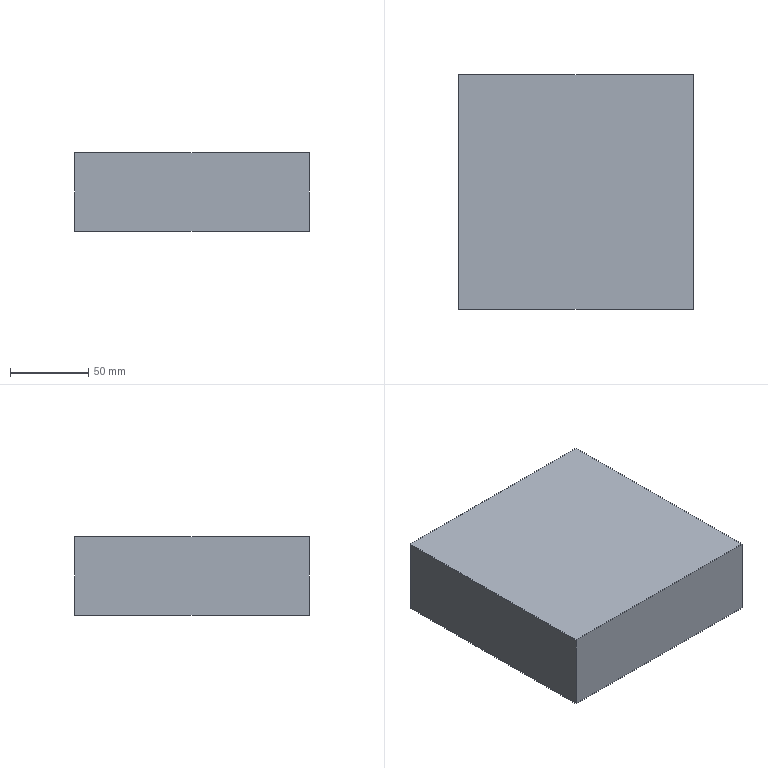Part | NX | features solid 2 | 1 solid | 6 faces | box 150 x 150 x 50 mm | volume 1125000 mm3 | plane 6
STEP:
#1=CARTESIAN_POINT('',(-1390.,-840.,-120.));
#2=VERTEX_POINT('',#1);
#3=CARTESIAN_POINT('',(-1240.,-840.,-120.));
#4=VERTEX_POINT('',#3);
#5=CARTESIAN_POINT('',(-1390.,-840.,-120.));
#6=DIRECTION('',(1.,0.,0.));
#7=VECTOR('',#6,1000.);
#8=LINE('',#5,#7);
#9=EDGE_CURVE('',#2,#4,#8,.T.);
#10=ORIENTED_EDGE('',*,*,#9,.F.);
#11=CARTESIAN_POINT('',(-1390.,-840.,-170.));
#12=VERTEX_POINT('',#11);
#13=CARTESIAN_POINT('',(-1390.,-840.,-170.));
#14=DIRECTION('',(0.,0.,1.));
#15=VECTOR('',#14,1000.);
#16=LINE('',#13,#15);
#17=EDGE_CURVE('',#12,#2,#16,.T.);
#18=ORIENTED_EDGE('',*,*,#17,.F.);
#19=CARTESIAN_POINT('',(-1240.,-840.,-170.));
#20=VERTEX_POINT('',#19);
#21=CARTESIAN_POINT('',(-1390.,-840.,-170.));
#22=DIRECTION('',(1.,0.,0.));
#23=VECTOR('',#22,1000.);
#24=LINE('',#21,#23);
#25=EDGE_CURVE('',#12,#20,#24,.T.);
#26=ORIENTED_EDGE('',*,*,#25,.T.);
#27=CARTESIAN_POINT('',(-1240.,-840.,-170.));
#28=DIRECTION('',(0.,0.,1.));
#29=VECTOR('',#28,1000.);
#30=LINE('',#27,#29);
#31=EDGE_CURVE('',#20,#4,#30,.T.);
#32=ORIENTED_EDGE('',*,*,#31,.T.);
#33=EDGE_LOOP('',(#10,#18,#26,#32));
#34=FACE_BOUND('',#33,.T.);
#35=CARTESIAN_POINT('',(-1390.,-840.,-170.));
#36=DIRECTION('',(0.,-1.,0.));
#37=DIRECTION('',(0.,0.,-1.));
#38=AXIS2_PLACEMENT_3D('',#35,#36,#37);
#39=PLANE('',#38);
#40=ADVANCED_FACE('',(#34),#39,.T.);
#41=CARTESIAN_POINT('',(-1240.,-690.,-120.));
#42=VERTEX_POINT('',#41);
#43=CARTESIAN_POINT('',(-1240.,-840.,-120.));
#44=DIRECTION('',(0.,1.,0.));
#45=VECTOR('',#44,1000.);
#46=LINE('',#43,#45);
#47=EDGE_CURVE('',#4,#42,#46,.T.);
#48=ORIENTED_EDGE('',*,*,#47,.F.);
#49=ORIENTED_EDGE('',*,*,#31,.F.);
#50=CARTESIAN_POINT('',(-1240.,-690.,-170.));
#51=VERTEX_POINT('',#50);
#52=CARTESIAN_POINT('',(-1240.,-840.,-170.));
#53=DIRECTION('',(0.,1.,0.));
#54=VECTOR('',#53,1000.);
#55=LINE('',#52,#54);
#56=EDGE_CURVE('',#20,#51,#55,.T.);
#57=ORIENTED_EDGE('',*,*,#56,.T.);
#58=CARTESIAN_POINT('',(-1240.,-690.,-170.));
#59=DIRECTION('',(0.,0.,1.));
#60=VECTOR('',#59,1000.);
#61=LINE('',#58,#60);
#62=EDGE_CURVE('',#51,#42,#61,.T.);
#63=ORIENTED_EDGE('',*,*,#62,.T.);
#64=EDGE_LOOP('',(#48,#49,#57,#63));
#65=FACE_BOUND('',#64,.T.);
#66=CARTESIAN_POINT('',(-1240.,-840.,-170.));
#67=DIRECTION('',(1.,0.,0.));
#68=DIRECTION('',(0.,0.,-1.));
#69=AXIS2_PLACEMENT_3D('',#66,#67,#68);
#70=PLANE('',#69);
#71=ADVANCED_FACE('',(#65),#70,.T.);
#72=CARTESIAN_POINT('',(-1390.,-690.,-120.));
#73=VERTEX_POINT('',#72);
#74=CARTESIAN_POINT('',(-1240.,-690.,-120.));
#75=DIRECTION('',(-1.,0.,0.));
#76=VECTOR('',#75,1000.);
#77=LINE('',#74,#76);
#78=EDGE_CURVE('',#42,#73,#77,.T.);
#79=ORIENTED_EDGE('',*,*,#78,.F.);
#80=ORIENTED_EDGE('',*,*,#62,.F.);
#81=CARTESIAN_POINT('',(-1390.,-690.,-170.));
#82=VERTEX_POINT('',#81);
#83=CARTESIAN_POINT('',(-1240.,-690.,-170.));
#84=DIRECTION('',(-1.,0.,0.));
#85=VECTOR('',#84,1000.);
#86=LINE('',#83,#85);
#87=EDGE_CURVE('',#51,#82,#86,.T.);
#88=ORIENTED_EDGE('',*,*,#87,.T.);
#89=CARTESIAN_POINT('',(-1390.,-690.,-170.));
#90=DIRECTION('',(0.,0.,1.));
#91=VECTOR('',#90,1000.);
#92=LINE('',#89,#91);
#93=EDGE_CURVE('',#82,#73,#92,.T.);
#94=ORIENTED_EDGE('',*,*,#93,.T.);
#95=EDGE_LOOP('',(#79,#80,#88,#94));
#96=FACE_BOUND('',#95,.T.);
#97=CARTESIAN_POINT('',(-1240.,-690.,-170.));
#98=DIRECTION('',(0.,1.,0.));
#99=DIRECTION('',(0.,0.,1.));
#100=AXIS2_PLACEMENT_3D('',#97,#98,#99);
#101=PLANE('',#100);
#102=ADVANCED_FACE('',(#96),#101,.T.);
#103=CARTESIAN_POINT('',(-1390.,-690.,-120.));
#104=DIRECTION('',(0.,-1.,0.));
#105=VECTOR('',#104,1000.);
#106=LINE('',#103,#105);
#107=EDGE_CURVE('',#73,#2,#106,.T.);
#108=ORIENTED_EDGE('',*,*,#107,.F.);
#109=ORIENTED_EDGE('',*,*,#93,.F.);
#110=CARTESIAN_POINT('',(-1390.,-690.,-170.));
#111=DIRECTION('',(0.,-1.,0.));
#112=VECTOR('',#111,1000.);
#113=LINE('',#110,#112);
#114=EDGE_CURVE('',#82,#12,#113,.T.);
#115=ORIENTED_EDGE('',*,*,#114,.T.);
#116=ORIENTED_EDGE('',*,*,#17,.T.);
#117=EDGE_LOOP('',(#108,#109,#115,#116));
#118=FACE_BOUND('',#117,.T.);
#119=CARTESIAN_POINT('',(-1390.,-690.,-170.));
#120=DIRECTION('',(-1.,0.,0.));
#121=DIRECTION('',(0.,0.,1.));
#122=AXIS2_PLACEMENT_3D('',#119,#120,#121);
#123=PLANE('',#122);
#124=ADVANCED_FACE('',(#118),#123,.T.);
#125=ORIENTED_EDGE('',*,*,#25,.F.);
#126=ORIENTED_EDGE('',*,*,#114,.F.);
#127=ORIENTED_EDGE('',*,*,#87,.F.);
#128=ORIENTED_EDGE('',*,*,#56,.F.);
#129=EDGE_LOOP('',(#125,#126,#127,#128));
#130=FACE_BOUND('',#129,.T.);
#131=CARTESIAN_POINT('',(-1240.,-840.,-170.));
#132=DIRECTION('',(0.,0.,1.));
#133=DIRECTION('',(1.,0.,0.));
#134=AXIS2_PLACEMENT_3D('',#131,#132,#133);
#135=PLANE('',#134);
#136=ADVANCED_FACE('',(#130),#135,.F.);
#137=ORIENTED_EDGE('',*,*,#9,.T.);
#138=ORIENTED_EDGE('',*,*,#47,.T.);
#139=ORIENTED_EDGE('',*,*,#78,.T.);
#140=ORIENTED_EDGE('',*,*,#107,.T.);
#141=EDGE_LOOP('',(#137,#138,#139,#140));
#142=FACE_BOUND('',#141,.T.);
#143=CARTESIAN_POINT('',(-1240.,-840.,-120.));
#144=DIRECTION('',(0.,0.,1.));
#145=DIRECTION('',(1.,0.,0.));
#146=AXIS2_PLACEMENT_3D('',#143,#144,#145);
#147=PLANE('',#146);
#148=ADVANCED_FACE('',(#142),#147,.T.);
#149=CLOSED_SHELL('',(#40,#71,#102,#124,#136,#148));
#150=MANIFOLD_SOLID_BREP('',#149);
#151=(LENGTH_UNIT()NAMED_UNIT(*)SI_UNIT(.MILLI.,.METRE.));
#152=UNCERTAINTY_MEASURE_WITH_UNIT(LENGTH_MEASURE(0.00001),#151,'','');
#153=(NAMED_UNIT(*)PLANE_ANGLE_UNIT()SI_UNIT($,.RADIAN.));
#154=(NAMED_UNIT(*)SI_UNIT($,.STERADIAN.)SOLID_ANGLE_UNIT());
#155=(GEOMETRIC_REPRESENTATION_CONTEXT(3)GLOBAL_UNCERTAINTY_ASSIGNED_CONTEXT((#152))GLOBAL_UNIT_ASSIGNED_CONTEXT((#151,#153,#154))REPRESENTATION_CONTEXT('',''));
#156=ADVANCED_BREP_SHAPE_REPRESENTATION('',(#150),#155);